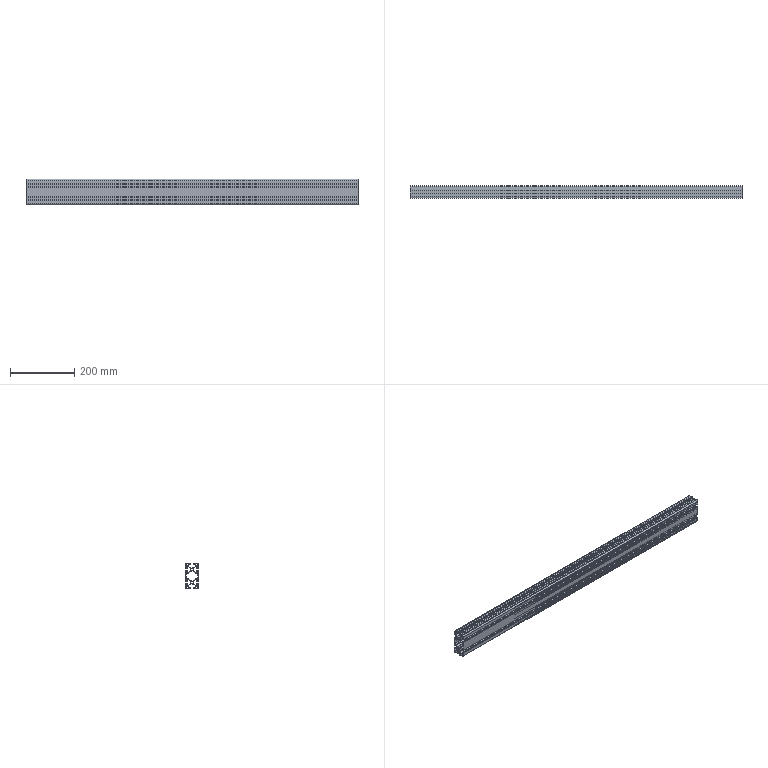Part | STEP file | 1 solid | 286 faces | box 1030 x 40 x 80 mm | volume 836128 mm3 | cylinder 144 | plane 142 | commonest cylinder face diameters 0.6 x44 2 x44 4 x28 0.4 x14 6 x4 6.8 x4